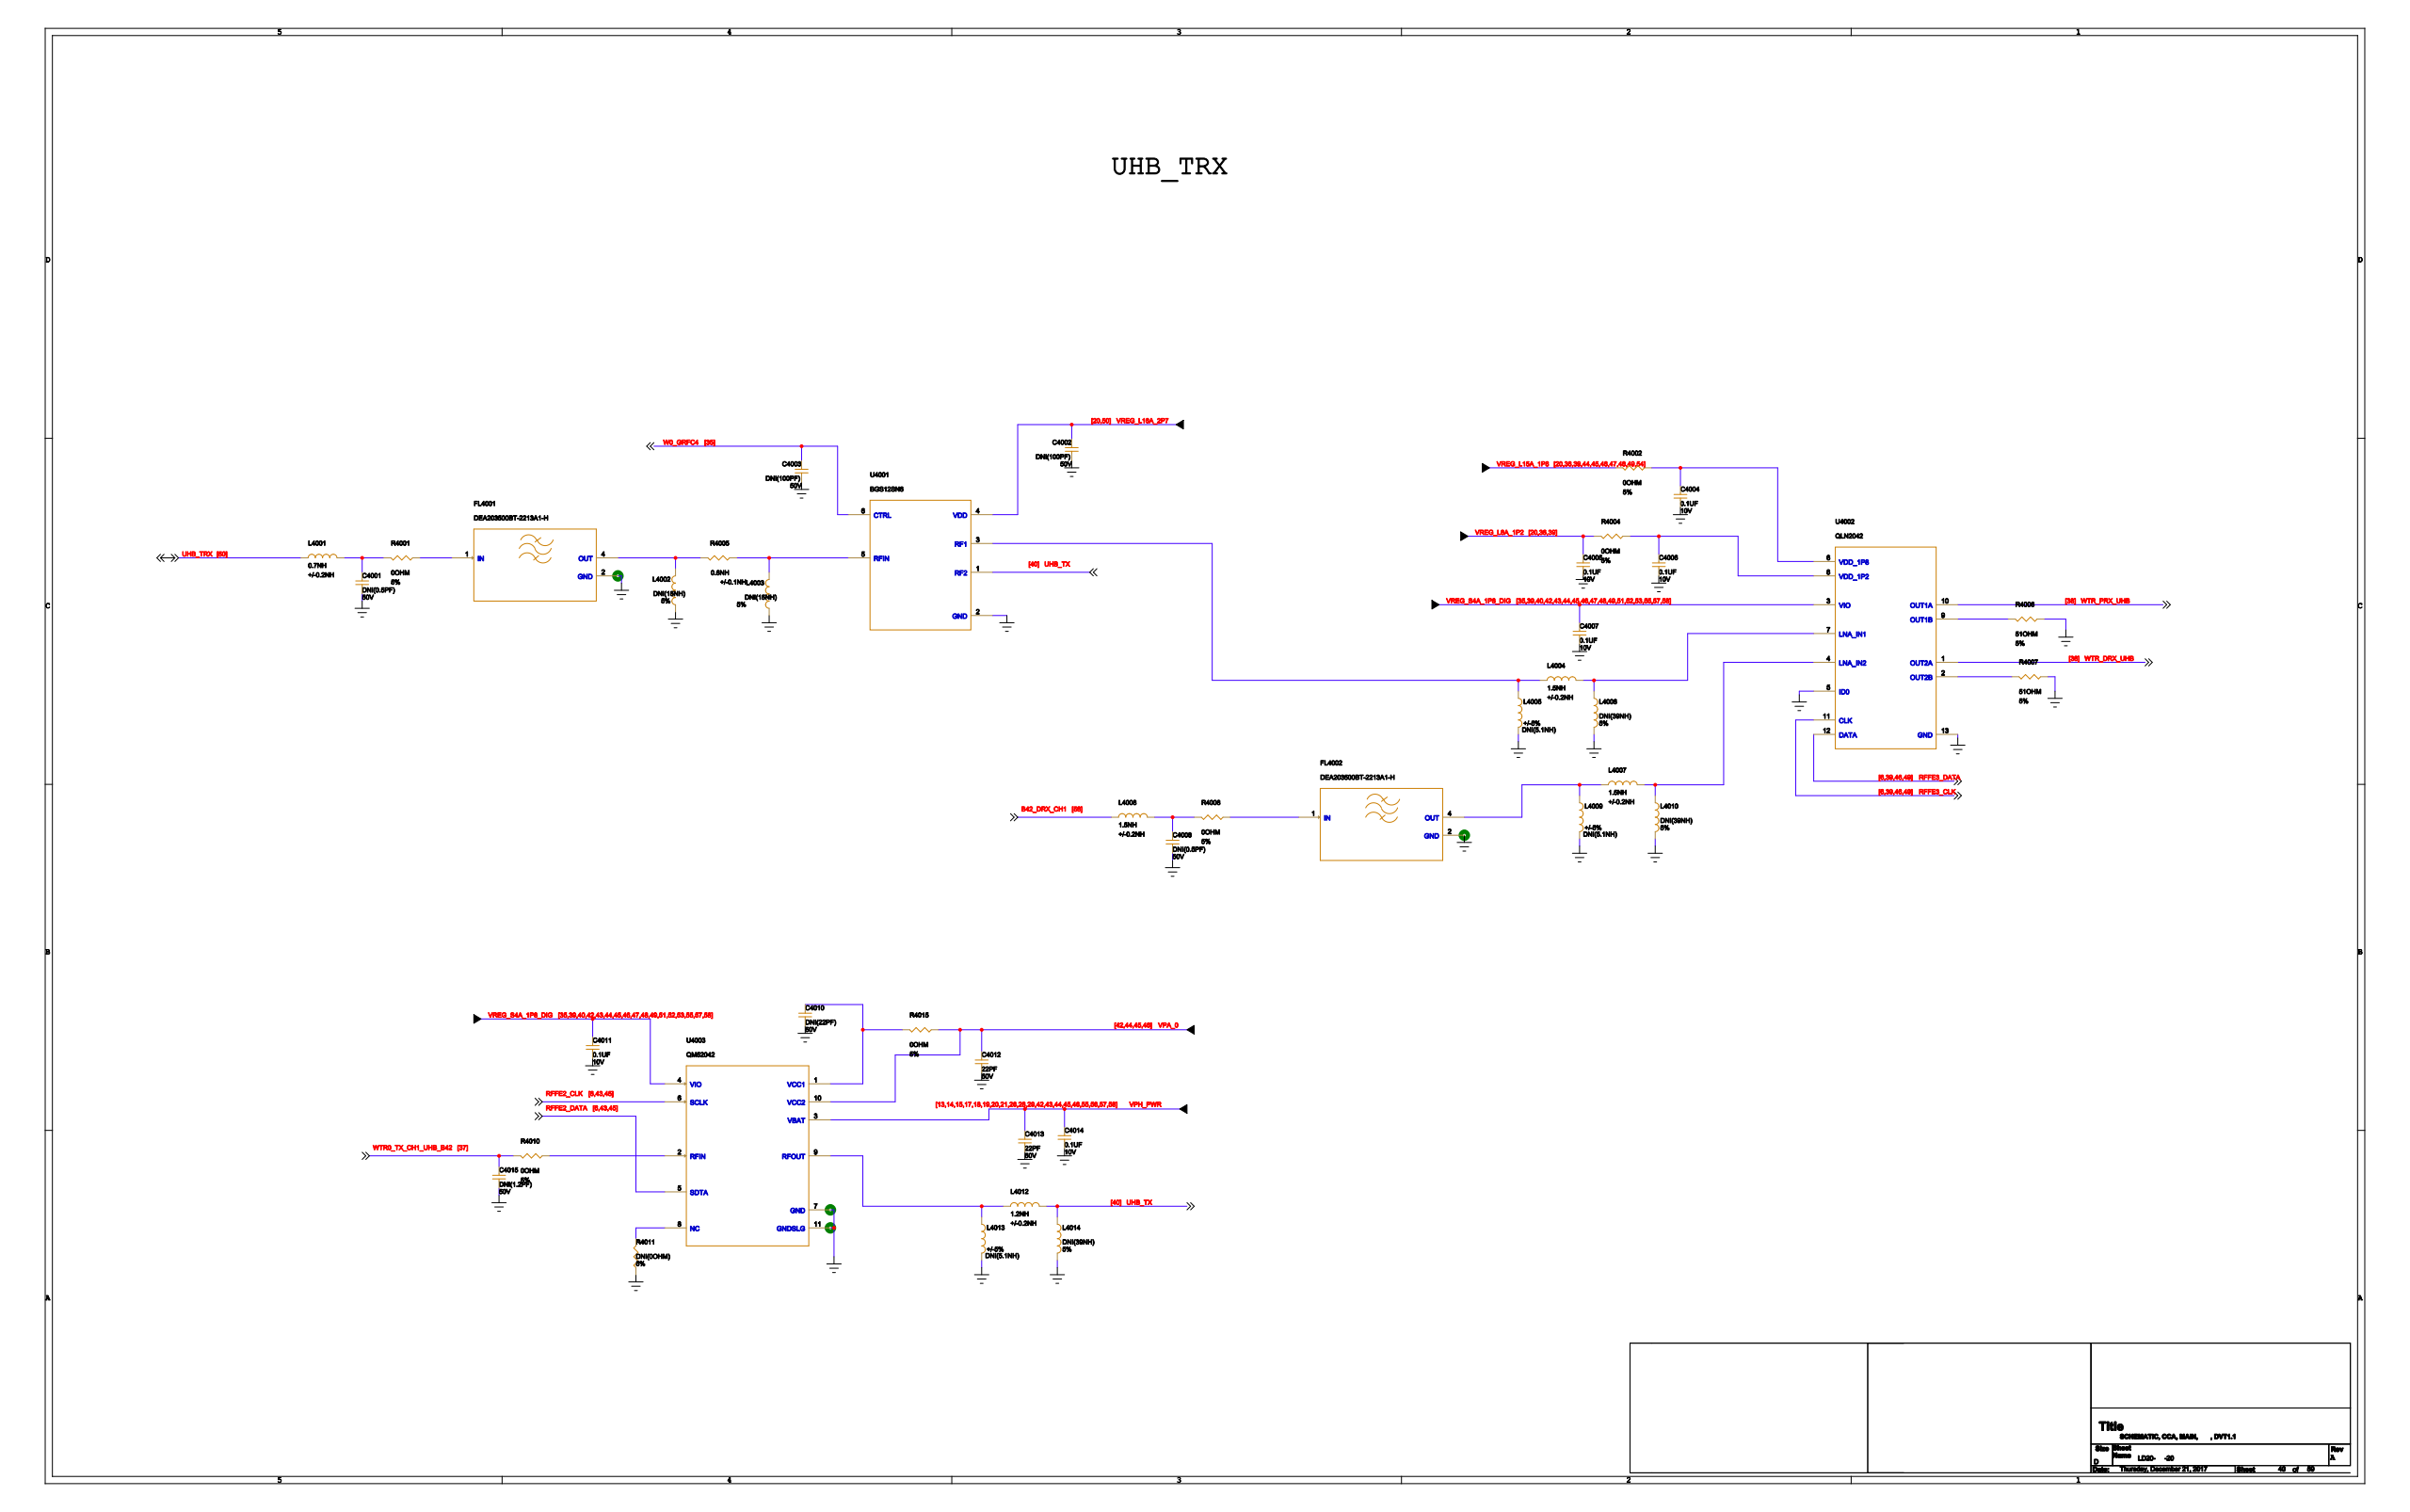Circuit board | Cadence Allegro | 1520 parts | 1149 nets | one sheet of the schematic
Parts on this sheet (reference | value | footprint):
C4001 | DNI(0.5PF) | 2P0201R_DNI
C4002 | DNI(100PF) | 2P0201R_DNI
C4003 | DNI(100PF) | 2P0201R_DNI
C4004 | 0.1UF | 2P0201R
C4005 | 0.1UF | 2P0201R
C4006 | 0.1UF | 2P0201R
C4007 | 0.1UF | 2P0201R
C4008 | DNI(0.5PF) | 2P0201R_DNI
C4010 | DNI(22PF) | 2P0201R_DNI
C4011 | 0.1UF | 2P0201R
C4012 | 22PF | 2P0201R
C4013 | 22PF | 2P0201R
C4014 | 0.1UF | 2P0201R
C4015 | DNI(1.2PF) | 2P0201R_DNI
FL4001 | DEA203500BT-2213A1-H | 3PSM85X53NV3
FL4002 | DEA203500BT-2213A1-H | 3PSM85X53NV3
L4001 | 0.7NH | 2P0201R
L4002 | DNI(15NH) | 2P0201R_DNI
L4003 | DNI(15NH) | 2P0201R_DNI
L4004 | 1.5NH | 2P0201R
L4005 | DNI(5.1NH) | 2P0201R_DNI
L4006 | DNI(39NH) | 2P0201R_DNI
L4007 | 1.5NH | 2P0201R
L4008 | 1.5NH | 2P0201R
L4009 | DNI(5.1NH) | 2P0201R_DNI
L4010 | DNI(39NH) | 2P0201R_DNI
L4012 | 1.2NH | 2P0201R
L4013 | DNI(5.1NH) | 2P0201R_DNI
L4014 | DNI(39NH) | 2P0201R_DNI
R4001 | 0OHM | 2P0201R
R4002 | 0OHM | 2P0201R
R4004 | 0OHM | 2P0201R
R4005 | 0.6NH | 2P0201R
R4006 | 51OHM | 2P0201R
R4007 | 51OHM | 2P0201R
R4008 | 0OHM | 2P0201R
R4010 | 0OHM | 2P0201R
R4011 | DNI(0OHM) | 2P0201R_DNI
R4015 | 0OHM | 2P0201R
U4001 | BGS12SN6 | 6PSM45X30N157
U4002 | QLN2042 | 13LGA79X81N
U4003 | QM52042 | 11PSM102X83N199V2
Nets of these parts (net: part-pin ...):
GND: C4001-2 C4002-2 C4003-2 C4004-2 C4005-2 C4006-2 C4007-2 C4008-2 C4010-2 C4011-2 C4012-2 C4013-2 C4014-2 C4015-2 FL4001-2 FL4002-2 L4002-2 L4003-2 L4005-2 L4006-2 L4009-2 L4010-2 L4013-2 L4014-2 R4006-2 R4007-2 R4011-2 U4001-2 U4002-5 U4002-13 U4003-7 U4003-11
N48231308: C4001-1 L4001-2 R4001-1
N48230925: C4008-1 L4008-2 R4008-1
WTR0_TX_CH1_UHB_B42: C4015-1 R4010-1
UHB_TRX: L4001-1
N48223745: FL4001-4 L4002-1 R4005-2
N48223743: L4003-1 R4005-1 U4001-5
N48231522: L4012-1 L4013-1 U4003-9
UHB_TX: L4012-2 L4014-1 U4001-1
VPA_0: C4012-1 R4015-2 U4003-10
RFFE2_CLK: U4003-6
RFFE2_DATA: U4003-5
VREG_L15A_1P8: R4002-1
VPH_PWR: C4013-1 C4014-1 U4003-3
N48227004: L4004-1 L4005-1 U4001-3
N48227420: FL4002-4 L4007-1 L4009-1
N48227022: L4004-2 L4006-1 U4002-7
N48227432: L4007-2 L4010-1 U4002-4
VREG_S4A_1P8_DIG: C4007-1 C4011-1 U4002-3 U4003-4
N48225445: C4010-1 R4015-1 U4003-1
N48231310: FL4001-1 R4001-2
N48231137: FL4002-1 R4008-2
B42_DRX_CH1: L4008-1
W0_GRFC4: C4003-1 U4001-6
VREG_L8A_1P2: C4005-1 R4004-1
WTR_DRX_UHB: U4002-1
WTR_PRX_UHB: U4002-10
VREG_L16A_2P7: C4002-1 U4001-4
RFFE3_CLK: U4002-11
RFFE3_DATA: U4002-12
N48229145: R4006-1 U4002-9
N48229133: R4007-1 U4002-2
N48226107: C4006-1 R4004-2 U4002-8
N48226138: C4004-1 R4002-2 U4002-6
N48224752: R4011-1 U4003-8
N48224668: R4010-2 U4003-2